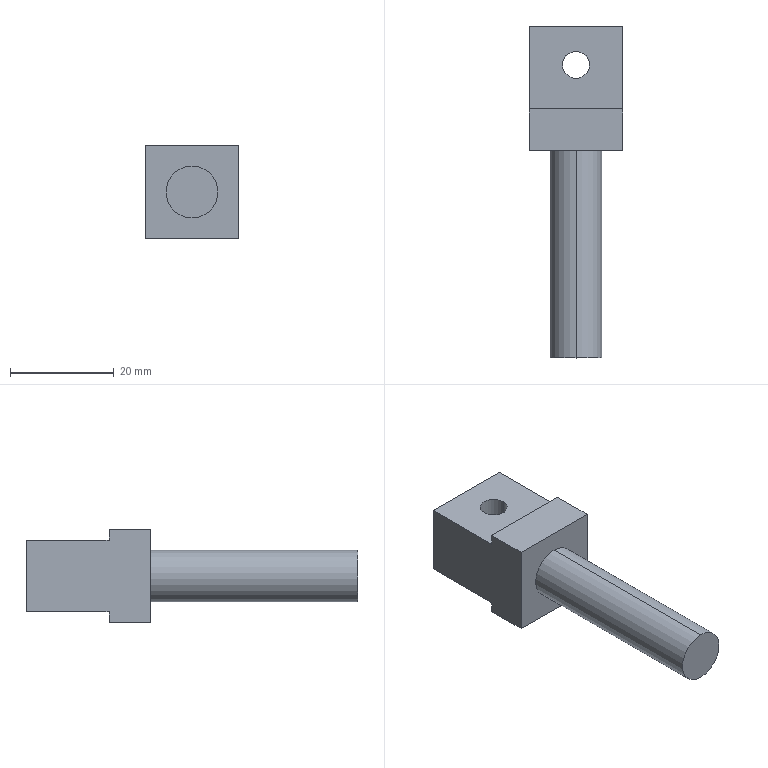Part | STEP file | PN_0003 (hook) | 1 solid | 15 faces | box 18 x 64 x 18 mm | volume 9415 mm3 | plane 11 | cylinder 4 | commonest cylinder face diameters 5.2 x2 10 x2
STEP:
#1=CARTESIAN_POINT('',(0.,0.,0.));
#2=DIRECTION('',(0.,0.,1.));
#3=DIRECTION('',(1.,0.,0.));
#4=AXIS2_PLACEMENT_3D('',#1,#2,#3);
#5=CARTESIAN_POINT('',(2.6,56.5,-6.9));
#6=VERTEX_POINT('',#5);
#7=CARTESIAN_POINT('',(2.6,56.5,6.9));
#8=VERTEX_POINT('',#7);
#9=CARTESIAN_POINT('',(2.6,56.5,-14.));
#10=DIRECTION('',(0.,0.,1.));
#11=VECTOR('',#10,1.);
#12=LINE('',#9,#11);
#13=CARTESIAN_POINT('',(0.,56.5,-14.));
#14=DIRECTION('',(0.,0.,1.));
#15=DIRECTION('',(1.,0.,0.));
#16=AXIS2_PLACEMENT_3D('',#13,#14,#15);
#17=CYLINDRICAL_SURFACE('',#16,2.6);
#18=CARTESIAN_POINT('',(6.283,0.));
#19=DIRECTION('',(0.,1.));
#20=VECTOR('',#19,1.);
#21=LINE('',#18,#20);
#22=(GEOMETRIC_REPRESENTATION_CONTEXT(2)PARAMETRIC_REPRESENTATION_CONTEXT()REPRESENTATION_CONTEXT('',''));
#23=DEFINITIONAL_REPRESENTATION('',(#21),#22);
#24=PCURVE('',#17,#23);
#25=CARTESIAN_POINT('',(0.,56.5,-14.));
#26=DIRECTION('',(0.,0.,1.));
#27=DIRECTION('',(1.,0.,0.));
#28=AXIS2_PLACEMENT_3D('',#25,#26,#27);
#29=CYLINDRICAL_SURFACE('',#28,2.6);
#30=CARTESIAN_POINT('',(0.,0.));
#31=DIRECTION('',(0.,1.));
#32=VECTOR('',#31,1.);
#33=LINE('',#30,#32);
#34=(GEOMETRIC_REPRESENTATION_CONTEXT(2)PARAMETRIC_REPRESENTATION_CONTEXT()REPRESENTATION_CONTEXT('',''));
#35=DEFINITIONAL_REPRESENTATION('',(#33),#34);
#36=PCURVE('',#29,#35);
#37=SURFACE_CURVE('',#12,(#24,#36),.PCURVE_S1.);
#38=EDGE_CURVE('',#6,#8,#37,.T.);
#39=ORIENTED_EDGE('',*,*,#38,.T.);
#40=CARTESIAN_POINT('',(-2.6,56.5,6.9));
#41=VERTEX_POINT('',#40);
#42=CARTESIAN_POINT('',(0.,56.5,6.9));
#43=DIRECTION('',(0.,0.,1.));
#44=DIRECTION('',(1.,0.,0.));
#45=AXIS2_PLACEMENT_3D('',#42,#43,#44);
#46=CIRCLE('',#45,2.6);
#47=CARTESIAN_POINT('',(0.,20.9));
#48=DIRECTION('',(1.,0.));
#49=VECTOR('',#48,1.);
#50=LINE('',#47,#49);
#51=(GEOMETRIC_REPRESENTATION_CONTEXT(2)PARAMETRIC_REPRESENTATION_CONTEXT()REPRESENTATION_CONTEXT('',''));
#52=DEFINITIONAL_REPRESENTATION('',(#50),#51);
#53=PCURVE('',#17,#52);
#54=CARTESIAN_POINT('',(-31.479,48.,6.9));
#55=DIRECTION('',(0.,0.,-1.));
#56=DIRECTION('',(-1.,0.,0.));
#57=AXIS2_PLACEMENT_3D('',#54,#55,#56);
#58=PLANE('',#57);
#59=CARTESIAN_POINT('',(-34.079,8.5));
#60=CARTESIAN_POINT('',(-34.079,13.003));
#61=CARTESIAN_POINT('',(-30.179,10.752));
#62=CARTESIAN_POINT('',(-26.279,8.5));
#63=CARTESIAN_POINT('',(-30.179,6.248));
#64=CARTESIAN_POINT('',(-34.079,3.997));
#65=CARTESIAN_POINT('',(-34.079,8.5));
#66=(BOUNDED_CURVE()B_SPLINE_CURVE(2,(#59,#60,#61,#62,#63,#64,#65),.UNSPECIFIED.,.T.,.F.)B_SPLINE_CURVE_WITH_KNOTS((1,2,2,2,2,1),(-2.094,0.,2.094,4.189,6.283,8.378),.UNSPECIFIED.)CURVE()GEOMETRIC_REPRESENTATION_ITEM()RATIONAL_B_SPLINE_CURVE((1.,0.5,1.,0.5,1.,0.5,1.))REPRESENTATION_ITEM(''));
#67=(GEOMETRIC_REPRESENTATION_CONTEXT(2)PARAMETRIC_REPRESENTATION_CONTEXT()REPRESENTATION_CONTEXT('',''));
#68=DEFINITIONAL_REPRESENTATION('',(#66),#67);
#69=PCURVE('',#58,#68);
#70=SURFACE_CURVE('',#46,(#53,#69),.PCURVE_S1.);
#71=EDGE_CURVE('',#41,#8,#70,.T.);
#72=ORIENTED_EDGE('',*,*,#71,.F.);
#73=CARTESIAN_POINT('',(-2.6,56.5,-6.9));
#74=VERTEX_POINT('',#73);
#75=CARTESIAN_POINT('',(-2.6,56.5,-14.));
#76=DIRECTION('',(0.,0.,1.));
#77=VECTOR('',#76,1.);
#78=LINE('',#75,#77);
#79=CARTESIAN_POINT('',(3.142,0.));
#80=DIRECTION('',(0.,1.));
#81=VECTOR('',#80,1.);
#82=LINE('',#79,#81);
#83=(GEOMETRIC_REPRESENTATION_CONTEXT(2)PARAMETRIC_REPRESENTATION_CONTEXT()REPRESENTATION_CONTEXT('',''));
#84=DEFINITIONAL_REPRESENTATION('',(#82),#83);
#85=PCURVE('',#17,#84);
#86=CARTESIAN_POINT('',(3.142,0.));
#87=DIRECTION('',(0.,1.));
#88=VECTOR('',#87,1.);
#89=LINE('',#86,#88);
#90=(GEOMETRIC_REPRESENTATION_CONTEXT(2)PARAMETRIC_REPRESENTATION_CONTEXT()REPRESENTATION_CONTEXT('',''));
#91=DEFINITIONAL_REPRESENTATION('',(#89),#90);
#92=PCURVE('',#29,#91);
#93=SURFACE_CURVE('',#78,(#85,#92),.PCURVE_S1.);
#94=EDGE_CURVE('',#74,#41,#93,.T.);
#95=ORIENTED_EDGE('',*,*,#94,.F.);
#96=CARTESIAN_POINT('',(0.,56.5,-6.9));
#97=DIRECTION('',(0.,0.,1.));
#98=DIRECTION('',(1.,0.,0.));
#99=AXIS2_PLACEMENT_3D('',#96,#97,#98);
#100=CIRCLE('',#99,2.6);
#101=CARTESIAN_POINT('',(0.,7.1));
#102=DIRECTION('',(1.,0.));
#103=VECTOR('',#102,1.);
#104=LINE('',#101,#103);
#105=(GEOMETRIC_REPRESENTATION_CONTEXT(2)PARAMETRIC_REPRESENTATION_CONTEXT()REPRESENTATION_CONTEXT('',''));
#106=DEFINITIONAL_REPRESENTATION('',(#104),#105);
#107=PCURVE('',#17,#106);
#108=CARTESIAN_POINT('',(-31.479,48.,-6.9));
#109=DIRECTION('',(0.,0.,1.));
#110=DIRECTION('',(1.,0.,0.));
#111=AXIS2_PLACEMENT_3D('',#108,#109,#110);
#112=PLANE('',#111);
#113=CARTESIAN_POINT('',(31.479,8.5));
#114=DIRECTION('',(1.,0.));
#115=AXIS2_PLACEMENT_2D('',#113,#114);
#116=CIRCLE('',#115,2.6);
#117=(GEOMETRIC_REPRESENTATION_CONTEXT(2)PARAMETRIC_REPRESENTATION_CONTEXT()REPRESENTATION_CONTEXT('',''));
#118=DEFINITIONAL_REPRESENTATION('',(#116),#117);
#119=PCURVE('',#112,#118);
#120=SURFACE_CURVE('',#100,(#107,#119),.PCURVE_S1.);
#121=EDGE_CURVE('',#74,#6,#120,.T.);
#122=ORIENTED_EDGE('',*,*,#121,.T.);
#123=EDGE_LOOP('',(#39,#72,#95,#122));
#124=FACE_BOUND('',#123,.F.);
#125=ADVANCED_FACE('',(#124),#17,.F.);
#126=CARTESIAN_POINT('',(0.,40.,-5.));
#127=VERTEX_POINT('',#126);
#128=CARTESIAN_POINT('',(0.,40.,5.));
#129=VERTEX_POINT('',#128);
#130=CARTESIAN_POINT('',(0.,40.,0.));
#131=DIRECTION('',(0.,-1.,0.));
#132=DIRECTION('',(0.,0.,-1.));
#133=AXIS2_PLACEMENT_3D('',#130,#131,#132);
#134=CIRCLE('',#133,5.);
#135=CARTESIAN_POINT('',(0.,0.,0.));
#136=DIRECTION('',(0.,-1.,0.));
#137=DIRECTION('',(0.,0.,-1.));
#138=AXIS2_PLACEMENT_3D('',#135,#136,#137);
#139=CYLINDRICAL_SURFACE('',#138,5.);
#140=CARTESIAN_POINT('',(0.,-40.));
#141=DIRECTION('',(1.,0.));
#142=VECTOR('',#141,1.);
#143=LINE('',#140,#142);
#144=(GEOMETRIC_REPRESENTATION_CONTEXT(2)PARAMETRIC_REPRESENTATION_CONTEXT()REPRESENTATION_CONTEXT('',''));
#145=DEFINITIONAL_REPRESENTATION('',(#143),#144);
#146=PCURVE('',#139,#145);
#147=CARTESIAN_POINT('',(5.,40.,0.));
#148=DIRECTION('',(0.,-1.,0.));
#149=DIRECTION('',(0.,0.,-1.));
#150=AXIS2_PLACEMENT_3D('',#147,#148,#149);
#151=PLANE('',#150);
#152=CARTESIAN_POINT('',(0.,-5.));
#153=DIRECTION('',(1.,0.));
#154=AXIS2_PLACEMENT_2D('',#152,#153);
#155=CIRCLE('',#154,5.);
#156=(GEOMETRIC_REPRESENTATION_CONTEXT(2)PARAMETRIC_REPRESENTATION_CONTEXT()REPRESENTATION_CONTEXT('',''));
#157=DEFINITIONAL_REPRESENTATION('',(#155),#156);
#158=PCURVE('',#151,#157);
#159=SURFACE_CURVE('',#134,(#146,#158),.PCURVE_S1.);
#160=EDGE_CURVE('',#127,#129,#159,.T.);
#161=ORIENTED_EDGE('',*,*,#160,.T.);
#162=CARTESIAN_POINT('',(0.,0.,5.));
#163=VERTEX_POINT('',#162);
#164=CARTESIAN_POINT('',(0.,0.,5.));
#165=DIRECTION('',(0.,-1.,0.));
#166=VECTOR('',#165,1.);
#167=LINE('',#164,#166);
#168=CARTESIAN_POINT('',(3.142,0.));
#169=DIRECTION('',(0.,1.));
#170=VECTOR('',#169,1.);
#171=LINE('',#168,#170);
#172=(GEOMETRIC_REPRESENTATION_CONTEXT(2)PARAMETRIC_REPRESENTATION_CONTEXT()REPRESENTATION_CONTEXT('',''));
#173=DEFINITIONAL_REPRESENTATION('',(#171),#172);
#174=PCURVE('',#139,#173);
#175=CARTESIAN_POINT('',(0.,0.,0.));
#176=DIRECTION('',(0.,-1.,0.));
#177=DIRECTION('',(0.,0.,-1.));
#178=AXIS2_PLACEMENT_3D('',#175,#176,#177);
#179=CYLINDRICAL_SURFACE('',#178,5.);
#180=CARTESIAN_POINT('',(3.142,0.));
#181=DIRECTION('',(0.,1.));
#182=VECTOR('',#181,1.);
#183=LINE('',#180,#182);
#184=(GEOMETRIC_REPRESENTATION_CONTEXT(2)PARAMETRIC_REPRESENTATION_CONTEXT()REPRESENTATION_CONTEXT('',''));
#185=DEFINITIONAL_REPRESENTATION('',(#183),#184);
#186=PCURVE('',#179,#185);
#187=SURFACE_CURVE('',#167,(#174,#186),.PCURVE_S1.);
#188=EDGE_CURVE('',#129,#163,#187,.T.);
#189=ORIENTED_EDGE('',*,*,#188,.T.);
#190=CARTESIAN_POINT('',(0.,0.,-5.));
#191=VERTEX_POINT('',#190);
#192=CARTESIAN_POINT('',(0.,0.,0.));
#193=DIRECTION('',(0.,-1.,0.));
#194=DIRECTION('',(0.,0.,-1.));
#195=AXIS2_PLACEMENT_3D('',#192,#193,#194);
#196=CIRCLE('',#195,5.);
#197=CARTESIAN_POINT('',(0.,0.));
#198=DIRECTION('',(1.,0.));
#199=VECTOR('',#198,1.);
#200=LINE('',#197,#199);
#201=(GEOMETRIC_REPRESENTATION_CONTEXT(2)PARAMETRIC_REPRESENTATION_CONTEXT()REPRESENTATION_CONTEXT('',''));
#202=DEFINITIONAL_REPRESENTATION('',(#200),#201);
#203=PCURVE('',#139,#202);
#204=CARTESIAN_POINT('',(0.,0.,0.));
#205=DIRECTION('',(0.,-1.,0.));
#206=DIRECTION('',(0.,0.,-1.));
#207=AXIS2_PLACEMENT_3D('',#204,#205,#206);
#208=PLANE('',#207);
#209=CARTESIAN_POINT('',(0.,0.));
#210=DIRECTION('',(1.,0.));
#211=AXIS2_PLACEMENT_2D('',#209,#210);
#212=CIRCLE('',#211,5.);
#213=(GEOMETRIC_REPRESENTATION_CONTEXT(2)PARAMETRIC_REPRESENTATION_CONTEXT()REPRESENTATION_CONTEXT('',''));
#214=DEFINITIONAL_REPRESENTATION('',(#212),#213);
#215=PCURVE('',#208,#214);
#216=SURFACE_CURVE('',#196,(#203,#215),.PCURVE_S1.);
#217=EDGE_CURVE('',#191,#163,#216,.T.);
#218=ORIENTED_EDGE('',*,*,#217,.F.);
#219=CARTESIAN_POINT('',(0.,0.,-5.));
#220=DIRECTION('',(0.,-1.,0.));
#221=VECTOR('',#220,1.);
#222=LINE('',#219,#221);
#223=CARTESIAN_POINT('',(0.,0.));
#224=DIRECTION('',(0.,1.));
#225=VECTOR('',#224,1.);
#226=LINE('',#223,#225);
#227=(GEOMETRIC_REPRESENTATION_CONTEXT(2)PARAMETRIC_REPRESENTATION_CONTEXT()REPRESENTATION_CONTEXT('',''));
#228=DEFINITIONAL_REPRESENTATION('',(#226),#227);
#229=PCURVE('',#139,#228);
#230=CARTESIAN_POINT('',(6.283,0.));
#231=DIRECTION('',(0.,1.));
#232=VECTOR('',#231,1.);
#233=LINE('',#230,#232);
#234=(GEOMETRIC_REPRESENTATION_CONTEXT(2)PARAMETRIC_REPRESENTATION_CONTEXT()REPRESENTATION_CONTEXT('',''));
#235=DEFINITIONAL_REPRESENTATION('',(#233),#234);
#236=PCURVE('',#179,#235);
#237=SURFACE_CURVE('',#222,(#229,#236),.PCURVE_S1.);
#238=EDGE_CURVE('',#127,#191,#237,.T.);
#239=ORIENTED_EDGE('',*,*,#238,.F.);
#240=EDGE_LOOP('',(#161,#189,#218,#239));
#241=FACE_BOUND('',#240,.T.);
#242=ADVANCED_FACE('',(#241),#139,.T.);
#243=ORIENTED_EDGE('',*,*,#217,.T.);
#244=CARTESIAN_POINT('',(0.,0.,0.));
#245=DIRECTION('',(0.,-1.,0.));
#246=DIRECTION('',(0.,0.,-1.));
#247=AXIS2_PLACEMENT_3D('',#244,#245,#246);
#248=CIRCLE('',#247,5.);
#249=CARTESIAN_POINT('',(0.,0.));
#250=DIRECTION('',(1.,0.));
#251=AXIS2_PLACEMENT_2D('',#249,#250);
#252=CIRCLE('',#251,5.);
#253=(GEOMETRIC_REPRESENTATION_CONTEXT(2)PARAMETRIC_REPRESENTATION_CONTEXT()REPRESENTATION_CONTEXT('',''));
#254=DEFINITIONAL_REPRESENTATION('',(#252),#253);
#255=PCURVE('',#208,#254);
#256=CARTESIAN_POINT('',(0.,0.));
#257=DIRECTION('',(1.,0.));
#258=VECTOR('',#257,1.);
#259=LINE('',#256,#258);
#260=(GEOMETRIC_REPRESENTATION_CONTEXT(2)PARAMETRIC_REPRESENTATION_CONTEXT()REPRESENTATION_CONTEXT('',''));
#261=DEFINITIONAL_REPRESENTATION('',(#259),#260);
#262=PCURVE('',#179,#261);
#263=SURFACE_CURVE('',#248,(#255,#262),.PCURVE_S1.);
#264=EDGE_CURVE('',#163,#191,#263,.T.);
#265=ORIENTED_EDGE('',*,*,#264,.T.);
#266=EDGE_LOOP('',(#243,#265));
#267=FACE_BOUND('',#266,.T.);
#268=ADVANCED_FACE('',(#267),#208,.T.);
#269=ORIENTED_EDGE('',*,*,#188,.F.);
#270=CARTESIAN_POINT('',(0.,40.,0.));
#271=DIRECTION('',(0.,-1.,0.));
#272=DIRECTION('',(0.,0.,-1.));
#273=AXIS2_PLACEMENT_3D('',#270,#271,#272);
#274=CIRCLE('',#273,5.);
#275=CARTESIAN_POINT('',(0.,-40.));
#276=DIRECTION('',(1.,0.));
#277=VECTOR('',#276,1.);
#278=LINE('',#275,#277);
#279=(GEOMETRIC_REPRESENTATION_CONTEXT(2)PARAMETRIC_REPRESENTATION_CONTEXT()REPRESENTATION_CONTEXT('',''));
#280=DEFINITIONAL_REPRESENTATION('',(#278),#279);
#281=PCURVE('',#179,#280);
#282=CARTESIAN_POINT('',(0.,-5.));
#283=DIRECTION('',(1.,0.));
#284=AXIS2_PLACEMENT_2D('',#282,#283);
#285=CIRCLE('',#284,5.);
#286=(GEOMETRIC_REPRESENTATION_CONTEXT(2)PARAMETRIC_REPRESENTATION_CONTEXT()REPRESENTATION_CONTEXT('',''));
#287=DEFINITIONAL_REPRESENTATION('',(#285),#286);
#288=PCURVE('',#151,#287);
#289=SURFACE_CURVE('',#274,(#281,#288),.PCURVE_S1.);
#290=EDGE_CURVE('',#129,#127,#289,.T.);
#291=ORIENTED_EDGE('',*,*,#290,.T.);
#292=ORIENTED_EDGE('',*,*,#238,.T.);
#293=ORIENTED_EDGE('',*,*,#264,.F.);
#294=EDGE_LOOP('',(#269,#291,#292,#293));
#295=FACE_BOUND('',#294,.T.);
#296=ADVANCED_FACE('',(#295),#179,.T.);
#297=CARTESIAN_POINT('',(9.,40.,9.));
#298=VERTEX_POINT('',#297);
#299=CARTESIAN_POINT('',(9.,40.,-9.));
#300=VERTEX_POINT('',#299);
#301=CARTESIAN_POINT('',(9.,40.,0.));
#302=DIRECTION('',(0.,0.,-1.));
#303=VECTOR('',#302,1.);
#304=LINE('',#301,#303);
#305=CARTESIAN_POINT('',(0.,4.));
#306=DIRECTION('',(1.,0.));
#307=VECTOR('',#306,1.);
#308=LINE('',#305,#307);
#309=(GEOMETRIC_REPRESENTATION_CONTEXT(2)PARAMETRIC_REPRESENTATION_CONTEXT()REPRESENTATION_CONTEXT('',''));
#310=DEFINITIONAL_REPRESENTATION('',(#308),#309);
#311=PCURVE('',#151,#310);
#312=CARTESIAN_POINT('',(9.,0.,-14.742));
#313=DIRECTION('',(-1.,0.,0.));
#314=DIRECTION('',(0.,0.,1.));
#315=AXIS2_PLACEMENT_3D('',#312,#313,#314);
#316=PLANE('',#315);
#317=CARTESIAN_POINT('',(14.742,40.));
#318=DIRECTION('',(-1.,0.));
#319=VECTOR('',#318,1.);
#320=LINE('',#317,#319);
#321=(GEOMETRIC_REPRESENTATION_CONTEXT(2)PARAMETRIC_REPRESENTATION_CONTEXT()REPRESENTATION_CONTEXT('',''));
#322=DEFINITIONAL_REPRESENTATION('',(#320),#321);
#323=PCURVE('',#316,#322);
#324=SURFACE_CURVE('',#304,(#311,#323),.PCURVE_S1.);
#325=EDGE_CURVE('',#298,#300,#324,.T.);
#326=ORIENTED_EDGE('',*,*,#325,.F.);
#327=CARTESIAN_POINT('',(-9.,40.,9.));
#328=VERTEX_POINT('',#327);
#329=CARTESIAN_POINT('',(5.,40.,9.));
#330=DIRECTION('',(1.,0.,0.));
#331=VECTOR('',#330,1.);
#332=LINE('',#329,#331);
#333=CARTESIAN_POINT('',(-9.,0.));
#334=DIRECTION('',(0.,1.));
#335=VECTOR('',#334,1.);
#336=LINE('',#333,#335);
#337=(GEOMETRIC_REPRESENTATION_CONTEXT(2)PARAMETRIC_REPRESENTATION_CONTEXT()REPRESENTATION_CONTEXT('',''));
#338=DEFINITIONAL_REPRESENTATION('',(#336),#337);
#339=PCURVE('',#151,#338);
#340=CARTESIAN_POINT('',(-17.295,0.,9.));
#341=DIRECTION('',(0.,0.,-1.));
#342=DIRECTION('',(-1.,0.,0.));
#343=AXIS2_PLACEMENT_3D('',#340,#341,#342);
#344=PLANE('',#343);
#345=CARTESIAN_POINT('',(-22.295,40.));
#346=DIRECTION('',(-1.,0.));
#347=VECTOR('',#346,1.);
#348=LINE('',#345,#347);
#349=(GEOMETRIC_REPRESENTATION_CONTEXT(2)PARAMETRIC_REPRESENTATION_CONTEXT()REPRESENTATION_CONTEXT('',''));
#350=DEFINITIONAL_REPRESENTATION('',(#348),#349);
#351=PCURVE('',#344,#350);
#352=SURFACE_CURVE('',#332,(#339,#351),.PCURVE_S1.);
#353=EDGE_CURVE('',#328,#298,#352,.T.);
#354=ORIENTED_EDGE('',*,*,#353,.F.);
#355=CARTESIAN_POINT('',(-9.,40.,-9.));
#356=VERTEX_POINT('',#355);
#357=CARTESIAN_POINT('',(-9.,40.,0.));
#358=DIRECTION('',(0.,0.,1.));
#359=VECTOR('',#358,1.);
#360=LINE('',#357,#359);
#361=CARTESIAN_POINT('',(0.,-14.));
#362=DIRECTION('',(-1.,0.));
#363=VECTOR('',#362,1.);
#364=LINE('',#361,#363);
#365=(GEOMETRIC_REPRESENTATION_CONTEXT(2)PARAMETRIC_REPRESENTATION_CONTEXT()REPRESENTATION_CONTEXT('',''));
#366=DEFINITIONAL_REPRESENTATION('',(#364),#365);
#367=PCURVE('',#151,#366);
#368=CARTESIAN_POINT('',(-9.,0.,-14.742));
#369=DIRECTION('',(1.,0.,0.));
#370=DIRECTION('',(0.,0.,-1.));
#371=AXIS2_PLACEMENT_3D('',#368,#369,#370);
#372=PLANE('',#371);
#373=CARTESIAN_POINT('',(-14.742,40.));
#374=DIRECTION('',(-1.,0.));
#375=VECTOR('',#374,1.);
#376=LINE('',#373,#375);
#377=(GEOMETRIC_REPRESENTATION_CONTEXT(2)PARAMETRIC_REPRESENTATION_CONTEXT()REPRESENTATION_CONTEXT('',''));
#378=DEFINITIONAL_REPRESENTATION('',(#376),#377);
#379=PCURVE('',#372,#378);
#380=SURFACE_CURVE('',#360,(#367,#379),.PCURVE_S1.);
#381=EDGE_CURVE('',#356,#328,#380,.T.);
#382=ORIENTED_EDGE('',*,*,#381,.F.);
#383=CARTESIAN_POINT('',(5.,40.,-9.));
#384=DIRECTION('',(-1.,0.,0.));
#385=VECTOR('',#384,1.);
#386=LINE('',#383,#385);
#387=CARTESIAN_POINT('',(9.,0.));
#388=DIRECTION('',(0.,-1.));
#389=VECTOR('',#388,1.);
#390=LINE('',#387,#389);
#391=(GEOMETRIC_REPRESENTATION_CONTEXT(2)PARAMETRIC_REPRESENTATION_CONTEXT()REPRESENTATION_CONTEXT('',''));
#392=DEFINITIONAL_REPRESENTATION('',(#390),#391);
#393=PCURVE('',#151,#392);
#394=CARTESIAN_POINT('',(-17.295,0.,-9.));
#395=DIRECTION('',(0.,0.,1.));
#396=DIRECTION('',(1.,0.,0.));
#397=AXIS2_PLACEMENT_3D('',#394,#395,#396);
#398=PLANE('',#397);
#399=CARTESIAN_POINT('',(22.295,40.));
#400=DIRECTION('',(-1.,0.));
#401=VECTOR('',#400,1.);
#402=LINE('',#399,#401);
#403=(GEOMETRIC_REPRESENTATION_CONTEXT(2)PARAMETRIC_REPRESENTATION_CONTEXT()REPRESENTATION_CONTEXT('',''));
#404=DEFINITIONAL_REPRESENTATION('',(#402),#403);
#405=PCURVE('',#398,#404);
#406=SURFACE_CURVE('',#386,(#393,#405),.PCURVE_S1.);
#407=EDGE_CURVE('',#300,#356,#406,.T.);
#408=ORIENTED_EDGE('',*,*,#407,.F.);
#409=EDGE_LOOP('',(#326,#354,#382,#408));
#410=FACE_BOUND('',#409,.T.);
#411=ORIENTED_EDGE('',*,*,#160,.F.);
#412=ORIENTED_EDGE('',*,*,#290,.F.);
#413=EDGE_LOOP('',(#411,#412));
#414=FACE_BOUND('',#413,.T.);
#415=ADVANCED_FACE('',(#410,#414),#151,.T.);
#416=CARTESIAN_POINT('',(9.,64.,-6.9));
#417=VERTEX_POINT('',#416);
#418=CARTESIAN_POINT('',(9.,64.,6.9));
#419=VERTEX_POINT('',#418);
#420=CARTESIAN_POINT('',(9.,64.,-14.742));
#421=DIRECTION('',(0.,0.,1.));
#422=VECTOR('',#421,1.);
#423=LINE('',#420,#422);
#424=CARTESIAN_POINT('',(14.,64.,0.));
#425=DIRECTION('',(0.,1.,0.));
#426=DIRECTION('',(0.,0.,1.));
#427=AXIS2_PLACEMENT_3D('',#424,#425,#426);
#428=PLANE('',#427);
#429=CARTESIAN_POINT('',(-14.742,-5.));
#430=DIRECTION('',(1.,0.));
#431=VECTOR('',#430,1.);
#432=LINE('',#429,#431);
#433=(GEOMETRIC_REPRESENTATION_CONTEXT(2)PARAMETRIC_REPRESENTATION_CONTEXT()REPRESENTATION_CONTEXT('',''));
#434=DEFINITIONAL_REPRESENTATION('',(#432),#433);
#435=PCURVE('',#428,#434);
#436=CARTESIAN_POINT('',(0.,64.));
#437=DIRECTION('',(1.,0.));
#438=VECTOR('',#437,1.);
#439=LINE('',#436,#438);
#440=(GEOMETRIC_REPRESENTATION_CONTEXT(2)PARAMETRIC_REPRESENTATION_CONTEXT()REPRESENTATION_CONTEXT('',''));
#441=DEFINITIONAL_REPRESENTATION('',(#439),#440);
#442=PCURVE('',#316,#441);
#443=SURFACE_CURVE('',#423,(#435,#442),.PCURVE_S1.);
#444=EDGE_CURVE('',#417,#419,#443,.T.);
#445=ORIENTED_EDGE('',*,*,#444,.F.);
#446=CARTESIAN_POINT('',(-9.,64.,-6.9));
#447=VERTEX_POINT('',#446);
#448=CARTESIAN_POINT('',(14.,64.,-6.9));
#449=DIRECTION('',(1.,0.,0.));
#450=VECTOR('',#449,1.);
#451=LINE('',#448,#450);
#452=CARTESIAN_POINT('',(-6.9,0.));
#453=DIRECTION('',(0.,1.));
#454=VECTOR('',#453,1.);
#455=LINE('',#452,#454);
#456=(GEOMETRIC_REPRESENTATION_CONTEXT(2)PARAMETRIC_REPRESENTATION_CONTEXT()REPRESENTATION_CONTEXT('',''));
#457=DEFINITIONAL_REPRESENTATION('',(#455),#456);
#458=PCURVE('',#428,#457);
#459=CARTESIAN_POINT('',(45.479,16.));
#460=DIRECTION('',(1.,0.));
#461=VECTOR('',#460,1.);
#462=LINE('',#459,#461);
#463=(GEOMETRIC_REPRESENTATION_CONTEXT(2)PARAMETRIC_REPRESENTATION_CONTEXT()REPRESENTATION_CONTEXT('',''));
#464=DEFINITIONAL_REPRESENTATION('',(#462),#463);
#465=PCURVE('',#112,#464);
#466=SURFACE_CURVE('',#451,(#458,#465),.PCURVE_S1.);
#467=EDGE_CURVE('',#447,#417,#466,.T.);
#468=ORIENTED_EDGE('',*,*,#467,.F.);
#469=CARTESIAN_POINT('',(-9.,64.,6.9));
#470=VERTEX_POINT('',#469);
#471=CARTESIAN_POINT('',(-9.,64.,-14.742));
#472=DIRECTION('',(0.,0.,-1.));
#473=VECTOR('',#472,1.);
#474=LINE('',#471,#473);
#475=CARTESIAN_POINT('',(-14.742,-23.));
#476=DIRECTION('',(-1.,0.));
#477=VECTOR('',#476,1.);
#478=LINE('',#475,#477);
#479=(GEOMETRIC_REPRESENTATION_CONTEXT(2)PARAMETRIC_REPRESENTATION_CONTEXT()REPRESENTATION_CONTEXT('',''));
#480=DEFINITIONAL_REPRESENTATION('',(#478),#479);
#481=PCURVE('',#428,#480);
#482=CARTESIAN_POINT('',(0.,64.));
#483=DIRECTION('',(1.,0.));
#484=VECTOR('',#483,1.);
#485=LINE('',#482,#484);
#486=(GEOMETRIC_REPRESENTATION_CONTEXT(2)PARAMETRIC_REPRESENTATION_CONTEXT()REPRESENTATION_CONTEXT('',''));
#487=DEFINITIONAL_REPRESENTATION('',(#485),#486);
#488=PCURVE('',#372,#487);
#489=SURFACE_CURVE('',#474,(#481,#488),.PCURVE_S1.);
#490=EDGE_CURVE('',#470,#447,#489,.T.);
#491=ORIENTED_EDGE('',*,*,#490,.F.);
#492=CARTESIAN_POINT('',(14.,64.,6.9));
#493=DIRECTION('',(-1.,0.,0.));
#494=VECTOR('',#493,1.);
#495=LINE('',#492,#494);
#496=CARTESIAN_POINT('',(6.9,0.));
#497=DIRECTION('',(0.,-1.));
#498=VECTOR('',#497,1.);
#499=LINE('',#496,#498);
#500=(GEOMETRIC_REPRESENTATION_CONTEXT(2)PARAMETRIC_REPRESENTATION_CONTEXT()REPRESENTATION_CONTEXT('',''));
#501=DEFINITIONAL_REPRESENTATION('',(#499),#500);
#502=PCURVE('',#428,#501);
#503=CARTESIAN_POINT('',(-45.479,16.));
#504=DIRECTION('',(1.,0.));
#505=VECTOR('',#504,1.);
#506=LINE('',#503,#505);
#507=(GEOMETRIC_REPRESENTATION_CONTEXT(2)PARAMETRIC_REPRESENTATION_CONTEXT()REPRESENTATION_CONTEXT('',''));
#508=DEFINITIONAL_REPRESENTATION('',(#506),#507);
#509=PCURVE('',#58,#508);
#510=SURFACE_CURVE('',#495,(#502,#509),.PCURVE_S1.);
#511=EDGE_CURVE('',#419,#470,#510,.T.);
#512=ORIENTED_EDGE('',*,*,#511,.F.);
#513=EDGE_LOOP('',(#445,#468,#491,#512));
#514=FACE_BOUND('',#513,.T.);
#515=ADVANCED_FACE('',(#514),#428,.T.);
#516=CARTESIAN_POINT('',(0.,56.5,-6.9));
#517=DIRECTION('',(0.,0.,1.));
#518=DIRECTION('',(1.,0.,0.));
#519=AXIS2_PLACEMENT_3D('',#516,#517,#518);
#520=CIRCLE('',#519,2.6);
#521=CARTESIAN_POINT('',(31.479,8.5));
#522=DIRECTION('',(1.,0.));
#523=AXIS2_PLACEMENT_2D('',#521,#522);
#524=CIRCLE('',#523,2.6);
#525=(GEOMETRIC_REPRESENTATION_CONTEXT(2)PARAMETRIC_REPRESENTATION_CONTEXT()REPRESENTATION_CONTEXT('',''));
#526=DEFINITIONAL_REPRESENTATION('',(#524),#525);
#527=PCURVE('',#112,#526);
#528=CARTESIAN_POINT('',(0.,7.1));
#529=DIRECTION('',(1.,0.));
#530=VECTOR('',#529,1.);
#531=LINE('',#528,#530);
#532=(GEOMETRIC_REPRESENTATION_CONTEXT(2)PARAMETRIC_REPRESENTATION_CONTEXT()REPRESENTATION_CONTEXT('',''));
#533=DEFINITIONAL_REPRESENTATION('',(#531),#532);
#534=PCURVE('',#29,#533);
#535=SURFACE_CURVE('',#520,(#527,#534),.PCURVE_S1.);
#536=EDGE_CURVE('',#6,#74,#535,.T.);
#537=ORIENTED_EDGE('',*,*,#536,.T.);
#538=ORIENTED_EDGE('',*,*,#121,.T.);
#539=EDGE_LOOP('',(#537,#538));
#540=FACE_BOUND('',#539,.T.);
#541=ORIENTED_EDGE('',*,*,#467,.T.);
#542=CARTESIAN_POINT('',(9.,48.,-6.9));
#543=VERTEX_POINT('',#542);
#544=CARTESIAN_POINT('',(9.,48.,-6.9));
#545=DIRECTION('',(0.,-1.,0.));
#546=VECTOR('',#545,1.);
#547=LINE('',#544,#546);
#548=CARTESIAN_POINT('',(40.479,0.));
#549=DIRECTION('',(0.,-1.));
#550=VECTOR('',#549,1.);
#551=LINE('',#548,#550);
#552=(GEOMETRIC_REPRESENTATION_CONTEXT(2)PARAMETRIC_REPRESENTATION_CONTEXT()REPRESENTATION_CONTEXT('',''));
#553=DEFINITIONAL_REPRESENTATION('',(#551),#552);
#554=PCURVE('',#112,#553);
#555=CARTESIAN_POINT('',(7.842,48.));
#556=DIRECTION('',(0.,-1.));
#557=VECTOR('',#556,1.);
#558=LINE('',#555,#557);
#559=(GEOMETRIC_REPRESENTATION_CONTEXT(2)PARAMETRIC_REPRESENTATION_CONTEXT()REPRESENTATION_CONTEXT('',''));
#560=DEFINITIONAL_REPRESENTATION('',(#558),#559);
#561=PCURVE('',#316,#560);
#562=SURFACE_CURVE('',#547,(#554,#561),.PCURVE_S1.);
#563=EDGE_CURVE('',#417,#543,#562,.T.);
#564=ORIENTED_EDGE('',*,*,#563,.T.);
#565=CARTESIAN_POINT('',(-9.,48.,-6.9));
#566=VERTEX_POINT('',#565);
#567=CARTESIAN_POINT('',(-31.479,48.,-6.9));
#568=DIRECTION('',(1.,0.,0.));
#569=VECTOR('',#568,1.);
#570=LINE('',#567,#569);
#571=CARTESIAN_POINT('',(0.,0.));
#572=DIRECTION('',(1.,0.));
#573=VECTOR('',#572,1.);
#574=LINE('',#571,#573);
#575=(GEOMETRIC_REPRESENTATION_CONTEXT(2)PARAMETRIC_REPRESENTATION_CONTEXT()REPRESENTATION_CONTEXT('',''));
#576=DEFINITIONAL_REPRESENTATION('',(#574),#575);
#577=PCURVE('',#112,#576);
#578=CARTESIAN_POINT('',(0.,48.,0.));
#579=DIRECTION('',(0.,1.,0.));
#580=DIRECTION('',(0.,0.,1.));
#581=AXIS2_PLACEMENT_3D('',#578,#579,#580);
#582=PLANE('',#581);
#583=CARTESIAN_POINT('',(-6.9,-31.479));
#584=DIRECTION('',(0.,1.));
#585=VECTOR('',#584,1.);
#586=LINE('',#583,#585);
#587=(GEOMETRIC_REPRESENTATION_CONTEXT(2)PARAMETRIC_REPRESENTATION_CONTEXT()REPRESENTATION_CONTEXT('',''));
#588=DEFINITIONAL_REPRESENTATION('',(#586),#587);
#589=PCURVE('',#582,#588);
#590=SURFACE_CURVE('',#570,(#577,#589),.PCURVE_S1.);
#591=EDGE_CURVE('',#566,#543,#590,.T.);
#592=ORIENTED_EDGE('',*,*,#591,.F.);
#593=CARTESIAN_POINT('',(-9.,48.,-6.9));
#594=DIRECTION('',(0.,1.,0.));
#595=VECTOR('',#594,1.);
#596=LINE('',#593,#595);
#597=CARTESIAN_POINT('',(22.479,0.));
#598=DIRECTION('',(0.,1.));
#599=VECTOR('',#598,1.);
#600=LINE('',#597,#599);
#601=(GEOMETRIC_REPRESENTATION_CONTEXT(2)PARAMETRIC_REPRESENTATION_CONTEXT()REPRESENTATION_CONTEXT('',''));
#602=DEFINITIONAL_REPRESENTATION('',(#600),#601);
#603=PCURVE('',#112,#602);
#604=CARTESIAN_POINT('',(-7.842,48.));
#605=DIRECTION('',(0.,1.));
#606=VECTOR('',#605,1.);
#607=LINE('',#604,#606);
#608=(GEOMETRIC_REPRESENTATION_CONTEXT(2)PARAMETRIC_REPRESENTATION_CONTEXT()REPRESENTATION_CONTEXT('',''));
#609=DEFINITIONAL_REPRESENTATION('',(#607),#608);
#610=PCURVE('',#372,#609);
#611=SURFACE_CURVE('',#596,(#603,#610),.PCURVE_S1.);
#612=EDGE_CURVE('',#566,#447,#611,.T.);
#613=ORIENTED_EDGE('',*,*,#612,.T.);
#614=EDGE_LOOP('',(#541,#564,#592,#613));
#615=FACE_BOUND('',#614,.T.);
#616=ADVANCED_FACE('',(#540,#615),#112,.F.);
#617=CARTESIAN_POINT('',(9.,48.,-9.));
#618=VERTEX_POINT('',#617);
#619=CARTESIAN_POINT('',(9.,48.,0.));
#620=DIRECTION('',(0.,0.,1.));
#621=VECTOR('',#620,1.);
#622=LINE('',#619,#621);
#623=CARTESIAN_POINT('',(0.,9.));
#624=DIRECTION('',(1.,0.));
#625=VECTOR('',#624,1.);
#626=LINE('',#623,#625);
#627=(GEOMETRIC_REPRESENTATION_CONTEXT(2)PARAMETRIC_REPRESENTATION_CONTEXT()REPRESENTATION_CONTEXT('',''));
#628=DEFINITIONAL_REPRESENTATION('',(#626),#627);
#629=PCURVE('',#582,#628);
#630=CARTESIAN_POINT('',(14.742,48.));
#631=DIRECTION('',(1.,0.));
#632=VECTOR('',#631,1.);
#633=LINE('',#630,#632);
#634=(GEOMETRIC_REPRESENTATION_CONTEXT(2)PARAMETRIC_REPRESENTATION_CONTEXT()REPRESENTATION_CONTEXT('',''));
#635=DEFINITIONAL_REPRESENTATION('',(#633),#634);
#636=PCURVE('',#316,#635);
#637=SURFACE_CURVE('',#622,(#629,#636),.PCURVE_S1.);
#638=EDGE_CURVE('',#618,#543,#637,.T.);
#639=ORIENTED_EDGE('',*,*,#638,.F.);
#640=CARTESIAN_POINT('',(-9.,48.,-9.));
#641=VERTEX_POINT('',#640);
#642=CARTESIAN_POINT('',(0.,48.,-9.));
#643=DIRECTION('',(1.,0.,0.));
#644=VECTOR('',#643,1.);
#645=LINE('',#642,#644);
#646=CARTESIAN_POINT('',(-9.,0.));
#647=DIRECTION('',(0.,1.));
#648=VECTOR('',#647,1.);
#649=LINE('',#646,#648);
#650=(GEOMETRIC_REPRESENTATION_CONTEXT(2)PARAMETRIC_REPRESENTATION_CONTEXT()REPRESENTATION_CONTEXT('',''));
#651=DEFINITIONAL_REPRESENTATION('',(#649),#650);
#652=PCURVE('',#582,#651);
#653=CARTESIAN_POINT('',(17.295,48.));
#654=DIRECTION('',(1.,0.));
#655=VECTOR('',#654,1.);
#656=LINE('',#653,#655);
#657=(GEOMETRIC_REPRESENTATION_CONTEXT(2)PARAMETRIC_REPRESENTATION_CONTEXT()REPRESENTATION_CONTEXT('',''));
#658=DEFINITIONAL_REPRESENTATION('',(#656),#657);
#659=PCURVE('',#398,#658);
#660=SURFACE_CURVE('',#645,(#652,#659),.PCURVE_S1.);
#661=EDGE_CURVE('',#641,#618,#660,.T.);
#662=ORIENTED_EDGE('',*,*,#661,.F.);
#663=CARTESIAN_POINT('',(-9.,48.,0.));
#664=DIRECTION('',(0.,0.,-1.));
#665=VECTOR('',#664,1.);
#666=LINE('',#663,#665);
#667=CARTESIAN_POINT('',(0.,-9.));
#668=DIRECTION('',(-1.,0.));
#669=VECTOR('',#668,1.);
#670=LINE('',#667,#669);
#671=(GEOMETRIC_REPRESENTATION_CONTEXT(2)PARAMETRIC_REPRESENTATION_CONTEXT()REPRESENTATION_CONTEXT('',''));
#672=DEFINITIONAL_REPRESENTATION('',(#670),#671);
#673=PCURVE('',#582,#672);
#674=CARTESIAN_POINT('',(-14.742,48.));
#675=DIRECTION('',(1.,0.));
#676=VECTOR('',#675,1.);
#677=LINE('',#674,#676);
#678=(GEOMETRIC_REPRESENTATION_CONTEXT(2)PARAMETRIC_REPRESENTATION_CONTEXT()REPRESENTATION_CONTEXT('',''));
#679=DEFINITIONAL_REPRESENTATION('',(#677),#678);
#680=PCURVE('',#372,#679);
#681=SURFACE_CURVE('',#666,(#673,#680),.PCURVE_S1.);
#682=EDGE_CURVE('',#566,#641,#681,.T.);
#683=ORIENTED_EDGE('',*,*,#682,.F.);
#684=ORIENTED_EDGE('',*,*,#591,.T.);
#685=EDGE_LOOP('',(#639,#662,#683,#684));
#686=FACE_BOUND('',#685,.T.);
#687=ADVANCED_FACE('',(#686),#582,.T.);
#688=CARTESIAN_POINT('',(0.,56.5,6.9));
#689=DIRECTION('',(0.,0.,1.));
#690=DIRECTION('',(1.,0.,0.));
#691=AXIS2_PLACEMENT_3D('',#688,#689,#690);
#692=CIRCLE('',#691,2.6);
#693=CARTESIAN_POINT('',(-34.079,8.5));
#694=CARTESIAN_POINT('',(-34.079,13.003));
#695=CARTESIAN_POINT('',(-30.179,10.752));
#696=CARTESIAN_POINT('',(-26.279,8.5));
#697=CARTESIAN_POINT('',(-30.179,6.248));
#698=CARTESIAN_POINT('',(-34.079,3.997));
#699=CARTESIAN_POINT('',(-34.079,8.5));
#700=(BOUNDED_CURVE()B_SPLINE_CURVE(2,(#693,#694,#695,#696,#697,#698,#699),.UNSPECIFIED.,.T.,.F.)B_SPLINE_CURVE_WITH_KNOTS((1,2,2,2,2,1),(-2.094,0.,2.094,4.189,6.283,8.378),.UNSPECIFIED.)CURVE()GEOMETRIC_REPRESENTATION_ITEM()RATIONAL_B_SPLINE_CURVE((1.,0.5,1.,0.5,1.,0.5,1.))REPRESENTATION_ITEM(''));
#701=(GEOMETRIC_REPRESENTATION_CONTEXT(2)PARAMETRIC_REPRESENTATION_CONTEXT()REPRESENTATION_CONTEXT('',''));
#702=DEFINITIONAL_REPRESENTATION('',(#700),#701);
#703=PCURVE('',#58,#702);
#704=CARTESIAN_POINT('',(0.,20.9));
#705=DIRECTION('',(1.,0.));
#706=VECTOR('',#705,1.);
#707=LINE('',#704,#706);
#708=(GEOMETRIC_REPRESENTATION_CONTEXT(2)PARAMETRIC_REPRESENTATION_CONTEXT()REPRESENTATION_CONTEXT('',''));
#709=DEFINITIONAL_REPRESENTATION('',(#707),#708);
#710=PCURVE('',#29,#709);
#711=SURFACE_CURVE('',#692,(#703,#710),.PCURVE_S1.);
#712=EDGE_CURVE('',#8,#41,#711,.T.);
#713=ORIENTED_EDGE('',*,*,#712,.F.);
#714=ORIENTED_EDGE('',*,*,#71,.F.);
#715=EDGE_LOOP('',(#713,#714));
#716=FACE_BOUND('',#715,.T.);
#717=CARTESIAN_POINT('',(9.,48.,6.9));
#718=VERTEX_POINT('',#717);
#719=CARTESIAN_POINT('',(-9.,48.,6.9));
#720=VERTEX_POINT('',#719);
#721=CARTESIAN_POINT('',(-31.479,48.,6.9));
#722=DIRECTION('',(-1.,0.,0.));
#723=VECTOR('',#722,1.);
#724=LINE('',#721,#723);
#725=CARTESIAN_POINT('',(0.,0.));
#726=DIRECTION('',(1.,0.));
#727=VECTOR('',#726,1.);
#728=LINE('',#725,#727);
#729=(GEOMETRIC_REPRESENTATION_CONTEXT(2)PARAMETRIC_REPRESENTATION_CONTEXT()REPRESENTATION_CONTEXT('',''));
#730=DEFINITIONAL_REPRESENTATION('',(#728),#729);
#731=PCURVE('',#58,#730);
#732=CARTESIAN_POINT('',(0.,48.,0.));
#733=DIRECTION('',(0.,1.,0.));
#734=DIRECTION('',(0.,0.,1.));
#735=AXIS2_PLACEMENT_3D('',#732,#733,#734);
#736=PLANE('',#735);
#737=CARTESIAN_POINT('',(6.9,-31.479));
#738=DIRECTION('',(0.,-1.));
#739=VECTOR('',#738,1.);
#740=LINE('',#737,#739);
#741=(GEOMETRIC_REPRESENTATION_CONTEXT(2)PARAMETRIC_REPRESENTATION_CONTEXT()REPRESENTATION_CONTEXT('',''));
#742=DEFINITIONAL_REPRESENTATION('',(#740),#741);
#743=PCURVE('',#736,#742);
#744=SURFACE_CURVE('',#724,(#731,#743),.PCURVE_S1.);
#745=EDGE_CURVE('',#718,#720,#744,.T.);
#746=ORIENTED_EDGE('',*,*,#745,.F.);
#747=CARTESIAN_POINT('',(9.,48.,6.9));
#748=DIRECTION('',(0.,1.,0.));
#749=VECTOR('',#748,1.);
#750=LINE('',#747,#749);
#751=CARTESIAN_POINT('',(-40.479,0.));
#752=DIRECTION('',(0.,1.));
#753=VECTOR('',#752,1.);
#754=LINE('',#751,#753);
#755=(GEOMETRIC_REPRESENTATION_CONTEXT(2)PARAMETRIC_REPRESENTATION_CONTEXT()REPRESENTATION_CONTEXT('',''));
#756=DEFINITIONAL_REPRESENTATION('',(#754),#755);
#757=PCURVE('',#58,#756);
#758=CARTESIAN_POINT('',(21.642,48.));
#759=DIRECTION('',(0.,1.));
#760=VECTOR('',#759,1.);
#761=LINE('',#758,#760);
#762=(GEOMETRIC_REPRESENTATION_CONTEXT(2)PARAMETRIC_REPRESENTATION_CONTEXT()REPRESENTATION_CONTEXT('',''));
#763=DEFINITIONAL_REPRESENTATION('',(#761),#762);
#764=PCURVE('',#316,#763);
#765=SURFACE_CURVE('',#750,(#757,#764),.PCURVE_S1.);
#766=EDGE_CURVE('',#718,#419,#765,.T.);
#767=ORIENTED_EDGE('',*,*,#766,.T.);
#768=ORIENTED_EDGE('',*,*,#511,.T.);
#769=CARTESIAN_POINT('',(-9.,48.,6.9));
#770=DIRECTION('',(0.,-1.,0.));
#771=VECTOR('',#770,1.);
#772=LINE('',#769,#771);
#773=CARTESIAN_POINT('',(-22.479,0.));
#774=DIRECTION('',(0.,-1.));
#775=VECTOR('',#774,1.);
#776=LINE('',#773,#775);
#777=(GEOMETRIC_REPRESENTATION_CONTEXT(2)PARAMETRIC_REPRESENTATION_CONTEXT()REPRESENTATION_CONTEXT('',''));
#778=DEFINITIONAL_REPRESENTATION('',(#776),#777);
#779=PCURVE('',#58,#778);
#780=CARTESIAN_POINT('',(-21.642,48.));
#781=DIRECTION('',(0.,-1.));
#782=VECTOR('',#781,1.);
#783=LINE('',#780,#782);
#784=(GEOMETRIC_REPRESENTATION_CONTEXT(2)PARAMETRIC_REPRESENTATION_CONTEXT()REPRESENTATION_CONTEXT('',''));
#785=DEFINITIONAL_REPRESENTATION('',(#783),#784);
#786=PCURVE('',#372,#785);
#787=SURFACE_CURVE('',#772,(#779,#786),.PCURVE_S1.);
#788=EDGE_CURVE('',#470,#720,#787,.T.);
#789=ORIENTED_EDGE('',*,*,#788,.T.);
#790=EDGE_LOOP('',(#746,#767,#768,#789));
#791=FACE_BOUND('',#790,.T.);
#792=ADVANCED_FACE('',(#716,#791),#58,.F.);
#793=CARTESIAN_POINT('',(9.,48.,9.));
#794=VERTEX_POINT('',#793);
#795=CARTESIAN_POINT('',(9.,48.,0.));
#796=DIRECTION('',(0.,0.,1.));
#797=VECTOR('',#796,1.);
#798=LINE('',#795,#797);
#799=CARTESIAN_POINT('',(0.,9.));
#800=DIRECTION('',(1.,0.));
#801=VECTOR('',#800,1.);
#802=LINE('',#799,#801);
#803=(GEOMETRIC_REPRESENTATION_CONTEXT(2)PARAMETRIC_REPRESENTATION_CONTEXT()REPRESENTATION_CONTEXT('',''));
#804=DEFINITIONAL_REPRESENTATION('',(#802),#803);
#805=PCURVE('',#736,#804);
#806=CARTESIAN_POINT('',(14.742,48.));
#807=DIRECTION('',(1.,0.));
#808=VECTOR('',#807,1.);
#809=LINE('',#806,#808);
#810=(GEOMETRIC_REPRESENTATION_CONTEXT(2)PARAMETRIC_REPRESENTATION_CONTEXT()REPRESENTATION_CONTEXT('',''));
#811=DEFINITIONAL_REPRESENTATION('',(#809),#810);
#812=PCURVE('',#316,#811);
#813=SURFACE_CURVE('',#798,(#805,#812),.PCURVE_S1.);
#814=EDGE_CURVE('',#718,#794,#813,.T.);
#815=ORIENTED_EDGE('',*,*,#814,.F.);
#816=ORIENTED_EDGE('',*,*,#745,.T.);
#817=CARTESIAN_POINT('',(-9.,48.,9.));
#818=VERTEX_POINT('',#817);
#819=CARTESIAN_POINT('',(-9.,48.,0.));
#820=DIRECTION('',(0.,0.,-1.));
#821=VECTOR('',#820,1.);
#822=LINE('',#819,#821);
#823=CARTESIAN_POINT('',(0.,-9.));
#824=DIRECTION('',(-1.,0.));
#825=VECTOR('',#824,1.);
#826=LINE('',#823,#825);
#827=(GEOMETRIC_REPRESENTATION_CONTEXT(2)PARAMETRIC_REPRESENTATION_CONTEXT()REPRESENTATION_CONTEXT('',''));
#828=DEFINITIONAL_REPRESENTATION('',(#826),#827);
#829=PCURVE('',#736,#828);
#830=CARTESIAN_POINT('',(-14.742,48.));
#831=DIRECTION('',(1.,0.));
#832=VECTOR('',#831,1.);
#833=LINE('',#830,#832);
#834=(GEOMETRIC_REPRESENTATION_CONTEXT(2)PARAMETRIC_REPRESENTATION_CONTEXT()REPRESENTATION_CONTEXT('',''));
#835=DEFINITIONAL_REPRESENTATION('',(#833),#834);
#836=PCURVE('',#372,#835);
#837=SURFACE_CURVE('',#822,(#829,#836),.PCURVE_S1.);
#838=EDGE_CURVE('',#818,#720,#837,.T.);
#839=ORIENTED_EDGE('',*,*,#838,.F.);
#840=CARTESIAN_POINT('',(0.,48.,9.));
#841=DIRECTION('',(-1.,0.,0.));
#842=VECTOR('',#841,1.);
#843=LINE('',#840,#842);
#844=CARTESIAN_POINT('',(9.,0.));
#845=DIRECTION('',(0.,-1.));
#846=VECTOR('',#845,1.);
#847=LINE('',#844,#846);
#848=(GEOMETRIC_REPRESENTATION_CONTEXT(2)PARAMETRIC_REPRESENTATION_CONTEXT()REPRESENTATION_CONTEXT('',''));
#849=DEFINITIONAL_REPRESENTATION('',(#847),#848);
#850=PCURVE('',#736,#849);
#851=CARTESIAN_POINT('',(-17.295,48.));
#852=DIRECTION('',(1.,0.));
#853=VECTOR('',#852,1.);
#854=LINE('',#851,#853);
#855=(GEOMETRIC_REPRESENTATION_CONTEXT(2)PARAMETRIC_REPRESENTATION_CONTEXT()REPRESENTATION_CONTEXT('',''));
#856=DEFINITIONAL_REPRESENTATION('',(#854),#855);
#857=PCURVE('',#344,#856);
#858=SURFACE_CURVE('',#843,(#850,#857),.PCURVE_S1.);
#859=EDGE_CURVE('',#794,#818,#858,.T.);
#860=ORIENTED_EDGE('',*,*,#859,.F.);
#861=EDGE_LOOP('',(#815,#816,#839,#860));
#862=FACE_BOUND('',#861,.T.);
#863=ADVANCED_FACE('',(#862),#736,.T.);
#864=ORIENTED_EDGE('',*,*,#712,.F.);
#865=ORIENTED_EDGE('',*,*,#38,.F.);
#866=ORIENTED_EDGE('',*,*,#536,.T.);
#867=ORIENTED_EDGE('',*,*,#94,.T.);
#868=EDGE_LOOP('',(#864,#865,#866,#867));
#869=FACE_BOUND('',#868,.F.);
#870=ADVANCED_FACE('',(#869),#29,.F.);
#871=ORIENTED_EDGE('',*,*,#661,.T.);
#872=CARTESIAN_POINT('',(9.,0.,-9.));
#873=DIRECTION('',(0.,-1.,0.));
#874=VECTOR('',#873,1.);
#875=LINE('',#872,#874);
#876=CARTESIAN_POINT('',(26.295,0.));
#877=DIRECTION('',(0.,-1.));
#878=VECTOR('',#877,1.);
#879=LINE('',#876,#878);
#880=(GEOMETRIC_REPRESENTATION_CONTEXT(2)PARAMETRIC_REPRESENTATION_CONTEXT()REPRESENTATION_CONTEXT('',''));
#881=DEFINITIONAL_REPRESENTATION('',(#879),#880);
#882=PCURVE('',#398,#881);
#883=CARTESIAN_POINT('',(5.742,0.));
#884=DIRECTION('',(0.,-1.));
#885=VECTOR('',#884,1.);
#886=LINE('',#883,#885);
#887=(GEOMETRIC_REPRESENTATION_CONTEXT(2)PARAMETRIC_REPRESENTATION_CONTEXT()REPRESENTATION_CONTEXT('',''));
#888=DEFINITIONAL_REPRESENTATION('',(#886),#887);
#889=PCURVE('',#316,#888);
#890=SURFACE_CURVE('',#875,(#882,#889),.PCURVE_S1.);
#891=EDGE_CURVE('',#618,#300,#890,.T.);
#892=ORIENTED_EDGE('',*,*,#891,.T.);
#893=ORIENTED_EDGE('',*,*,#407,.T.);
#894=CARTESIAN_POINT('',(-9.,0.,-9.));
#895=DIRECTION('',(0.,1.,0.));
#896=VECTOR('',#895,1.);
#897=LINE('',#894,#896);
#898=CARTESIAN_POINT('',(8.295,0.));
#899=DIRECTION('',(0.,1.));
#900=VECTOR('',#899,1.);
#901=LINE('',#898,#900);
#902=(GEOMETRIC_REPRESENTATION_CONTEXT(2)PARAMETRIC_REPRESENTATION_CONTEXT()REPRESENTATION_CONTEXT('',''));
#903=DEFINITIONAL_REPRESENTATION('',(#901),#902);
#904=PCURVE('',#398,#903);
#905=CARTESIAN_POINT('',(-5.742,0.));
#906=DIRECTION('',(0.,1.));
#907=VECTOR('',#906,1.);
#908=LINE('',#905,#907);
#909=(GEOMETRIC_REPRESENTATION_CONTEXT(2)PARAMETRIC_REPRESENTATION_CONTEXT()REPRESENTATION_CONTEXT('',''));
#910=DEFINITIONAL_REPRESENTATION('',(#908),#909);
#911=PCURVE('',#372,#910);
#912=SURFACE_CURVE('',#897,(#904,#911),.PCURVE_S1.);
#913=EDGE_CURVE('',#356,#641,#912,.T.);
#914=ORIENTED_EDGE('',*,*,#913,.T.);
#915=EDGE_LOOP('',(#871,#892,#893,#914));
#916=FACE_BOUND('',#915,.T.);
#917=ADVANCED_FACE('',(#916),#398,.F.);
#918=ORIENTED_EDGE('',*,*,#353,.T.);
#919=CARTESIAN_POINT('',(9.,0.,9.));
#920=DIRECTION('',(0.,1.,0.));
#921=VECTOR('',#920,1.);
#922=LINE('',#919,#921);
#923=CARTESIAN_POINT('',(-26.295,0.));
#924=DIRECTION('',(0.,1.));
#925=VECTOR('',#924,1.);
#926=LINE('',#923,#925);
#927=(GEOMETRIC_REPRESENTATION_CONTEXT(2)PARAMETRIC_REPRESENTATION_CONTEXT()REPRESENTATION_CONTEXT('',''));
#928=DEFINITIONAL_REPRESENTATION('',(#926),#927);
#929=PCURVE('',#344,#928);
#930=CARTESIAN_POINT('',(23.742,0.));
#931=DIRECTION('',(0.,1.));
#932=VECTOR('',#931,1.);
#933=LINE('',#930,#932);
#934=(GEOMETRIC_REPRESENTATION_CONTEXT(2)PARAMETRIC_REPRESENTATION_CONTEXT()REPRESENTATION_CONTEXT('',''));
#935=DEFINITIONAL_REPRESENTATION('',(#933),#934);
#936=PCURVE('',#316,#935);
#937=SURFACE_CURVE('',#922,(#929,#936),.PCURVE_S1.);
#938=EDGE_CURVE('',#298,#794,#937,.T.);
#939=ORIENTED_EDGE('',*,*,#938,.T.);
#940=ORIENTED_EDGE('',*,*,#859,.T.);
#941=CARTESIAN_POINT('',(-9.,0.,9.));
#942=DIRECTION('',(0.,-1.,0.));
#943=VECTOR('',#942,1.);
#944=LINE('',#941,#943);
#945=CARTESIAN_POINT('',(-8.295,0.));
#946=DIRECTION('',(0.,-1.));
#947=VECTOR('',#946,1.);
#948=LINE('',#945,#947);
#949=(GEOMETRIC_REPRESENTATION_CONTEXT(2)PARAMETRIC_REPRESENTATION_CONTEXT()REPRESENTATION_CONTEXT('',''));
#950=DEFINITIONAL_REPRESENTATION('',(#948),#949);
#951=PCURVE('',#344,#950);
#952=CARTESIAN_POINT('',(-23.742,0.));
#953=DIRECTION('',(0.,-1.));
#954=VECTOR('',#953,1.);
#955=LINE('',#952,#954);
#956=(GEOMETRIC_REPRESENTATION_CONTEXT(2)PARAMETRIC_REPRESENTATION_CONTEXT()REPRESENTATION_CONTEXT('',''));
#957=DEFINITIONAL_REPRESENTATION('',(#955),#956);
#958=PCURVE('',#372,#957);
#959=SURFACE_CURVE('',#944,(#951,#958),.PCURVE_S1.);
#960=EDGE_CURVE('',#818,#328,#959,.T.);
#961=ORIENTED_EDGE('',*,*,#960,.T.);
#962=EDGE_LOOP('',(#918,#939,#940,#961));
#963=FACE_BOUND('',#962,.T.);
#964=ADVANCED_FACE('',(#963),#344,.F.);
#965=ORIENTED_EDGE('',*,*,#682,.T.);
#966=ORIENTED_EDGE('',*,*,#913,.F.);
#967=ORIENTED_EDGE('',*,*,#381,.T.);
#968=ORIENTED_EDGE('',*,*,#960,.F.);
#969=ORIENTED_EDGE('',*,*,#838,.T.);
#970=ORIENTED_EDGE('',*,*,#788,.F.);
#971=ORIENTED_EDGE('',*,*,#490,.T.);
#972=ORIENTED_EDGE('',*,*,#612,.F.);
#973=EDGE_LOOP('',(#965,#966,#967,#968,#969,#970,#971,#972));
#974=FACE_BOUND('',#973,.T.);
#975=ADVANCED_FACE('',(#974),#372,.F.);
#976=ORIENTED_EDGE('',*,*,#444,.T.);
#977=ORIENTED_EDGE('',*,*,#766,.F.);
#978=ORIENTED_EDGE('',*,*,#814,.T.);
#979=ORIENTED_EDGE('',*,*,#938,.F.);
#980=ORIENTED_EDGE('',*,*,#325,.T.);
#981=ORIENTED_EDGE('',*,*,#891,.F.);
#982=ORIENTED_EDGE('',*,*,#638,.T.);
#983=ORIENTED_EDGE('',*,*,#563,.F.);
#984=EDGE_LOOP('',(#976,#977,#978,#979,#980,#981,#982,#983));
#985=FACE_BOUND('',#984,.T.);
#986=ADVANCED_FACE('',(#985),#316,.F.);
#987=CLOSED_SHELL('',(#125,#242,#268,#296,#415,#515,#616,#687,#792,#863,#870,#917,#964,#975,#986));
#988=MANIFOLD_SOLID_BREP('',#987);
#989=(LENGTH_UNIT()NAMED_UNIT(*)SI_UNIT(.MILLI.,.METRE.));
#990=UNCERTAINTY_MEASURE_WITH_UNIT(LENGTH_MEASURE(0.0000001),#989,'','');
#991=(NAMED_UNIT(*)PLANE_ANGLE_UNIT()SI_UNIT($,.RADIAN.));
#992=(NAMED_UNIT(*)SI_UNIT($,.STERADIAN.)SOLID_ANGLE_UNIT());
#993=(GEOMETRIC_REPRESENTATION_CONTEXT(3)GLOBAL_UNCERTAINTY_ASSIGNED_CONTEXT((#990))GLOBAL_UNIT_ASSIGNED_CONTEXT((#989,#991,#992))REPRESENTATION_CONTEXT('',''));
#994=ADVANCED_BREP_SHAPE_REPRESENTATION('',(#4,#988),#993);